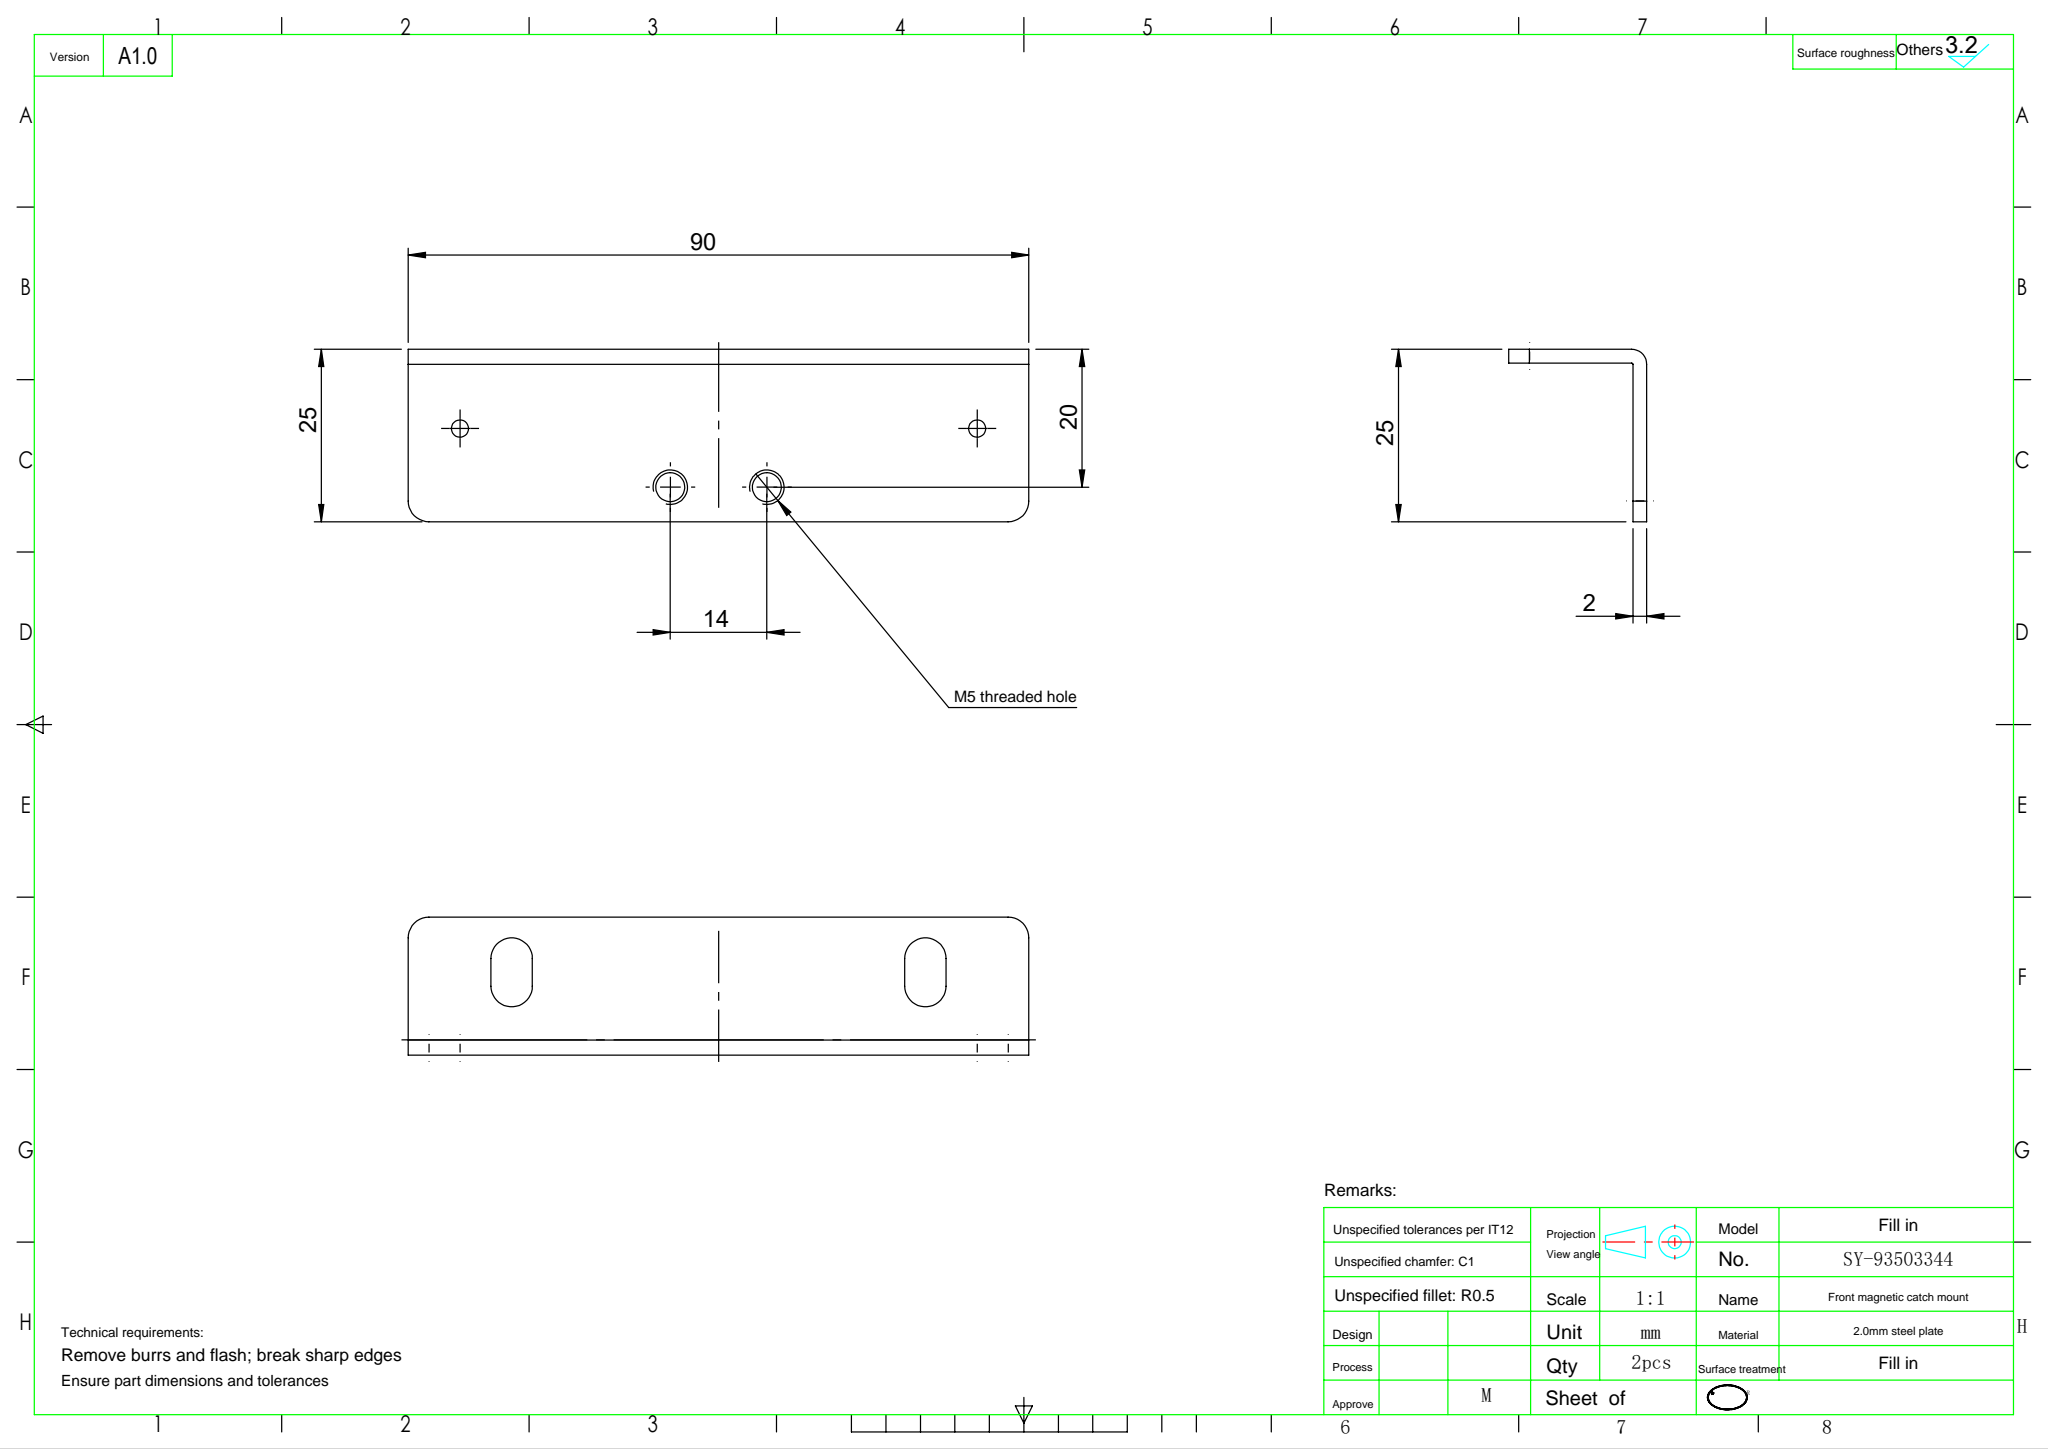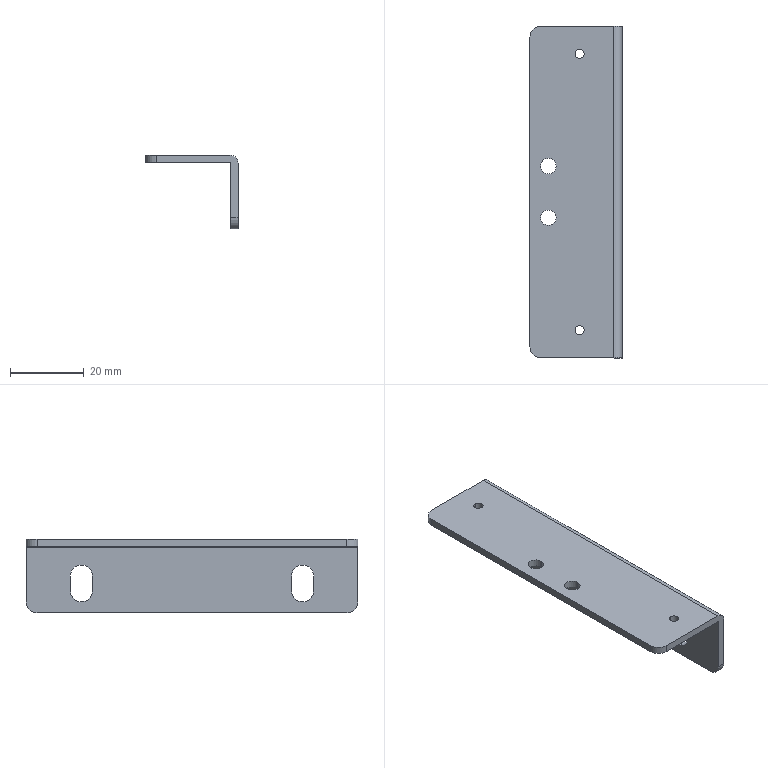Part | SolidWorks | features BaseBody 1, HoleWzd 1 | 1 solid | 32 faces | box 25 x 90 x 20 mm | volume 7348 mm3 | cylinder 20 | plane 12 | commonest cylinder face diameters 6 x10 2.5 x4 4.2 x4 0.4 x1 4.4 x1